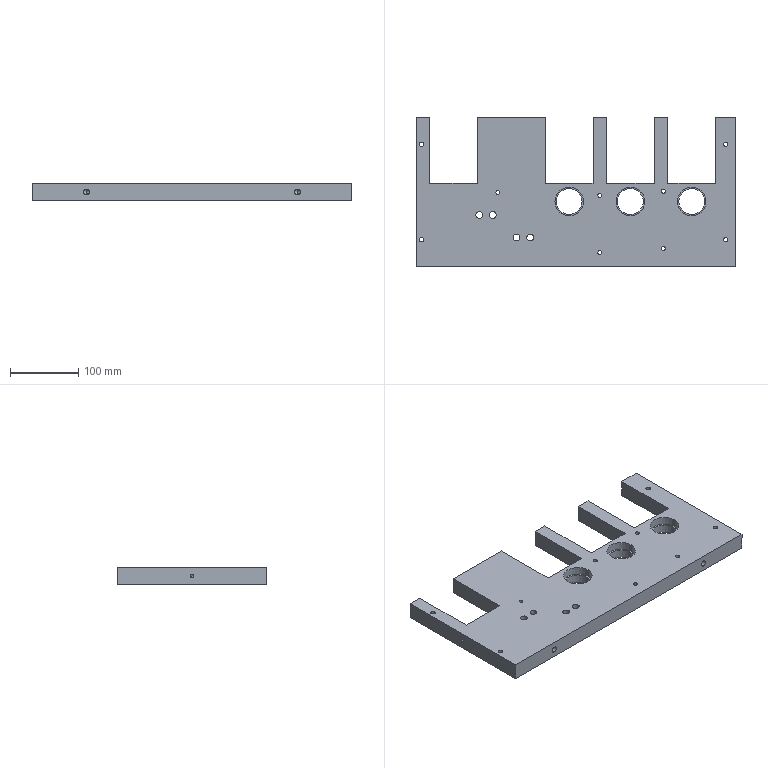Part | SolidWorks | features ICE 8, HoleWzd 3, Cut 2, 3DProfileFeature 1, Extrusion 1, LPattern 1 | 1 solid | 118 faces | box 470 x 220 x 25 mm | volume 1786055 mm3 | cylinder 68 | plane 30 | cone 20 | commonest cylinder face diameters 6.8 x12 10 x10 6 x8 6.5 x8 11 x8 38 x6